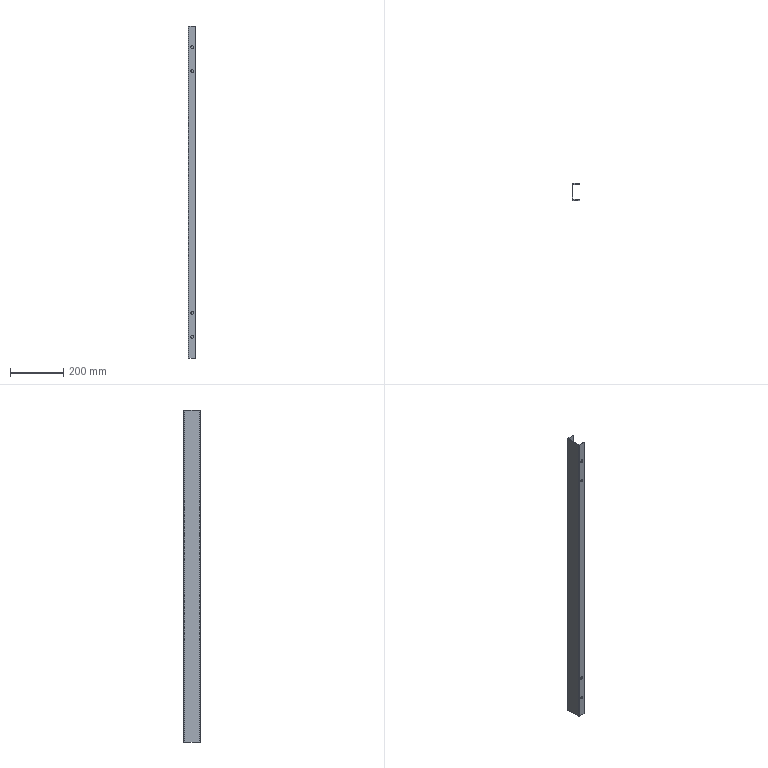Part | 1 solid | 59 faces | box 30 x 62 x 1250 mm | volume 424199 mm3 | cylinder 31 | plane 28 | commonest cylinder face diameters 10 x15 11 x8 4 x4 0.4 x2 6.4 x2